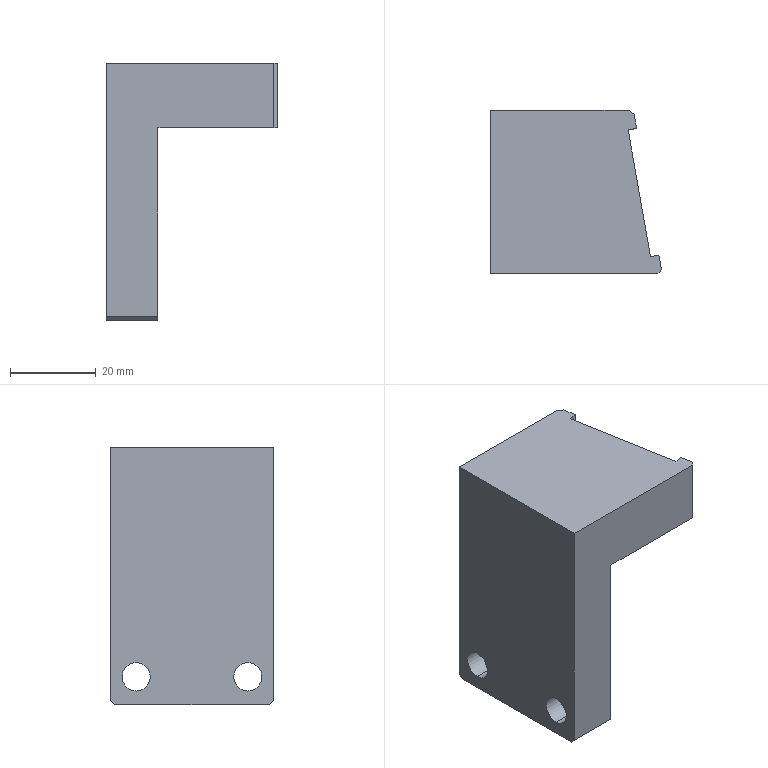Part | SolidWorks | features BaseBody 1 | 1 solid | 30 faces | box 39.85 x 38 x 60 mm | volume 38628 mm3 | plane 18 | cylinder 10 | cone 2 | commonest cylinder face diameters 6.6 x4 11 x4 5 x2
STEP:
#1=CARTESIAN_POINT('',(0.,6.,-56.8));
#2=VERTEX_POINT('',#1);
#3=CARTESIAN_POINT('',(0.,6.,-50.2));
#4=VERTEX_POINT('',#3);
#5=CARTESIAN_POINT('',(0.,6.,-53.5));
#6=DIRECTION('',(-1.,0.,0.));
#7=DIRECTION('',(0.,0.,-1.));
#8=AXIS2_PLACEMENT_3D('',#5,#6,#7);
#9=CIRCLE('',#8,3.3);
#10=EDGE_CURVE('',#2,#4,#9,.T.);
#11=ORIENTED_EDGE('',*,*,#10,.T.);
#12=CARTESIAN_POINT('',(6.,6.,-50.2));
#13=VERTEX_POINT('',#12);
#14=CARTESIAN_POINT('',(12.,6.,-50.2));
#15=DIRECTION('',(1.,0.,0.));
#16=VECTOR('',#15,1000.);
#17=LINE('',#14,#16);
#18=EDGE_CURVE('',#4,#13,#17,.T.);
#19=ORIENTED_EDGE('',*,*,#18,.T.);
#20=CARTESIAN_POINT('',(6.,6.,-56.8));
#21=VERTEX_POINT('',#20);
#22=CARTESIAN_POINT('',(6.,6.,-53.5));
#23=DIRECTION('',(-1.,0.,0.));
#24=DIRECTION('',(0.,0.,-1.));
#25=AXIS2_PLACEMENT_3D('',#22,#23,#24);
#26=CIRCLE('',#25,3.3);
#27=EDGE_CURVE('',#21,#13,#26,.T.);
#28=ORIENTED_EDGE('',*,*,#27,.F.);
#29=CARTESIAN_POINT('',(12.,6.,-56.8));
#30=DIRECTION('',(1.,0.,0.));
#31=VECTOR('',#30,1000.);
#32=LINE('',#29,#31);
#33=EDGE_CURVE('',#2,#21,#32,.T.);
#34=ORIENTED_EDGE('',*,*,#33,.F.);
#35=EDGE_LOOP('',(#11,#19,#28,#34));
#36=FACE_OUTER_BOUND('',#35,.T.);
#37=CARTESIAN_POINT('',(12.,6.,-53.5));
#38=DIRECTION('',(1.,0.,0.));
#39=DIRECTION('',(0.,0.,-1.));
#40=AXIS2_PLACEMENT_3D('',#37,#38,#39);
#41=CYLINDRICAL_SURFACE('',#40,3.3);
#42=ADVANCED_FACE('',(#36),#41,.F.);
#43=CARTESIAN_POINT('',(0.,32.,-56.8));
#44=VERTEX_POINT('',#43);
#45=CARTESIAN_POINT('',(0.,32.,-50.2));
#46=VERTEX_POINT('',#45);
#47=CARTESIAN_POINT('',(0.,32.,-53.5));
#48=DIRECTION('',(-1.,0.,0.));
#49=DIRECTION('',(0.,0.,-1.));
#50=AXIS2_PLACEMENT_3D('',#47,#48,#49);
#51=CIRCLE('',#50,3.3);
#52=EDGE_CURVE('',#44,#46,#51,.T.);
#53=ORIENTED_EDGE('',*,*,#52,.T.);
#54=CARTESIAN_POINT('',(6.,32.,-50.2));
#55=VERTEX_POINT('',#54);
#56=CARTESIAN_POINT('',(12.,32.,-50.2));
#57=DIRECTION('',(1.,0.,0.));
#58=VECTOR('',#57,1000.);
#59=LINE('',#56,#58);
#60=EDGE_CURVE('',#46,#55,#59,.T.);
#61=ORIENTED_EDGE('',*,*,#60,.T.);
#62=CARTESIAN_POINT('',(6.,32.,-56.8));
#63=VERTEX_POINT('',#62);
#64=CARTESIAN_POINT('',(6.,32.,-53.5));
#65=DIRECTION('',(-1.,0.,0.));
#66=DIRECTION('',(0.,0.,-1.));
#67=AXIS2_PLACEMENT_3D('',#64,#65,#66);
#68=CIRCLE('',#67,3.3);
#69=EDGE_CURVE('',#63,#55,#68,.T.);
#70=ORIENTED_EDGE('',*,*,#69,.F.);
#71=CARTESIAN_POINT('',(12.,32.,-56.8));
#72=DIRECTION('',(1.,0.,0.));
#73=VECTOR('',#72,1000.);
#74=LINE('',#71,#73);
#75=EDGE_CURVE('',#44,#63,#74,.T.);
#76=ORIENTED_EDGE('',*,*,#75,.F.);
#77=EDGE_LOOP('',(#53,#61,#70,#76));
#78=FACE_OUTER_BOUND('',#77,.T.);
#79=CARTESIAN_POINT('',(12.,32.,-53.5));
#80=DIRECTION('',(1.,0.,0.));
#81=DIRECTION('',(0.,0.,-1.));
#82=AXIS2_PLACEMENT_3D('',#79,#80,#81);
#83=CYLINDRICAL_SURFACE('',#82,3.3);
#84=ADVANCED_FACE('',(#78),#83,.F.);
#85=CARTESIAN_POINT('',(6.,6.,-59.));
#86=VERTEX_POINT('',#85);
#87=CARTESIAN_POINT('',(6.,6.,-48.));
#88=VERTEX_POINT('',#87);
#89=CARTESIAN_POINT('',(6.,6.,-53.5));
#90=DIRECTION('',(-1.,0.,0.));
#91=DIRECTION('',(0.,0.,-1.));
#92=AXIS2_PLACEMENT_3D('',#89,#90,#91);
#93=CIRCLE('',#92,5.5);
#94=EDGE_CURVE('',#86,#88,#93,.T.);
#95=ORIENTED_EDGE('',*,*,#94,.T.);
#96=CARTESIAN_POINT('',(12.,6.,-48.));
#97=VERTEX_POINT('',#96);
#98=CARTESIAN_POINT('',(12.,6.,-48.));
#99=DIRECTION('',(1.,0.,0.));
#100=VECTOR('',#99,1000.);
#101=LINE('',#98,#100);
#102=EDGE_CURVE('',#88,#97,#101,.T.);
#103=ORIENTED_EDGE('',*,*,#102,.T.);
#104=CARTESIAN_POINT('',(12.,6.,-59.));
#105=VERTEX_POINT('',#104);
#106=CARTESIAN_POINT('',(12.,6.,-53.5));
#107=DIRECTION('',(1.,0.,0.));
#108=DIRECTION('',(0.,0.,-1.));
#109=AXIS2_PLACEMENT_3D('',#106,#107,#108);
#110=CIRCLE('',#109,5.5);
#111=EDGE_CURVE('',#97,#105,#110,.T.);
#112=ORIENTED_EDGE('',*,*,#111,.T.);
#113=CARTESIAN_POINT('',(12.,6.,-59.));
#114=DIRECTION('',(1.,0.,0.));
#115=VECTOR('',#114,1000.);
#116=LINE('',#113,#115);
#117=EDGE_CURVE('',#86,#105,#116,.T.);
#118=ORIENTED_EDGE('',*,*,#117,.F.);
#119=EDGE_LOOP('',(#95,#103,#112,#118));
#120=FACE_OUTER_BOUND('',#119,.T.);
#121=CARTESIAN_POINT('',(12.,6.,-53.5));
#122=DIRECTION('',(1.,0.,0.));
#123=DIRECTION('',(0.,0.,-1.));
#124=AXIS2_PLACEMENT_3D('',#121,#122,#123);
#125=CYLINDRICAL_SURFACE('',#124,5.5);
#126=ADVANCED_FACE('',(#120),#125,.F.);
#127=CARTESIAN_POINT('',(6.,32.,-59.));
#128=VERTEX_POINT('',#127);
#129=CARTESIAN_POINT('',(6.,32.,-48.));
#130=VERTEX_POINT('',#129);
#131=CARTESIAN_POINT('',(6.,32.,-53.5));
#132=DIRECTION('',(-1.,0.,0.));
#133=DIRECTION('',(0.,0.,-1.));
#134=AXIS2_PLACEMENT_3D('',#131,#132,#133);
#135=CIRCLE('',#134,5.5);
#136=EDGE_CURVE('',#128,#130,#135,.T.);
#137=ORIENTED_EDGE('',*,*,#136,.T.);
#138=CARTESIAN_POINT('',(12.,32.,-48.));
#139=VERTEX_POINT('',#138);
#140=CARTESIAN_POINT('',(12.,32.,-48.));
#141=DIRECTION('',(1.,0.,0.));
#142=VECTOR('',#141,1000.);
#143=LINE('',#140,#142);
#144=EDGE_CURVE('',#130,#139,#143,.T.);
#145=ORIENTED_EDGE('',*,*,#144,.T.);
#146=CARTESIAN_POINT('',(12.,32.,-59.));
#147=VERTEX_POINT('',#146);
#148=CARTESIAN_POINT('',(12.,32.,-53.5));
#149=DIRECTION('',(1.,0.,0.));
#150=DIRECTION('',(0.,0.,-1.));
#151=AXIS2_PLACEMENT_3D('',#148,#149,#150);
#152=CIRCLE('',#151,5.5);
#153=EDGE_CURVE('',#139,#147,#152,.T.);
#154=ORIENTED_EDGE('',*,*,#153,.T.);
#155=CARTESIAN_POINT('',(12.,32.,-59.));
#156=DIRECTION('',(1.,0.,0.));
#157=VECTOR('',#156,1000.);
#158=LINE('',#155,#157);
#159=EDGE_CURVE('',#128,#147,#158,.T.);
#160=ORIENTED_EDGE('',*,*,#159,.F.);
#161=EDGE_LOOP('',(#137,#145,#154,#160));
#162=FACE_OUTER_BOUND('',#161,.T.);
#163=CARTESIAN_POINT('',(12.,32.,-53.5));
#164=DIRECTION('',(1.,0.,0.));
#165=DIRECTION('',(0.,0.,-1.));
#166=AXIS2_PLACEMENT_3D('',#163,#164,#165);
#167=CYLINDRICAL_SURFACE('',#166,5.5);
#168=ADVANCED_FACE('',(#162),#167,.F.);
#169=CARTESIAN_POINT('',(20.342,13.586,-7.5));
#170=VERTEX_POINT('',#169);
#171=CARTESIAN_POINT('',(19.474,18.51,-7.5));
#172=VERTEX_POINT('',#171);
#173=CARTESIAN_POINT('',(19.908,16.048,-7.5));
#174=DIRECTION('',(0.9848,0.1736,0.));
#175=DIRECTION('',(-0.1736,0.9848,0.));
#176=AXIS2_PLACEMENT_3D('',#173,#174,#175);
#177=CIRCLE('',#176,2.5);
#178=EDGE_CURVE('',#170,#172,#177,.T.);
#179=ORIENTED_EDGE('',*,*,#178,.F.);
#180=CARTESIAN_POINT('',(35.114,16.191,-7.5));
#181=VERTEX_POINT('',#180);
#182=CARTESIAN_POINT('',(35.114,16.191,-7.5));
#183=DIRECTION('',(0.9848,0.1736,0.));
#184=VECTOR('',#183,1000.);
#185=LINE('',#182,#184);
#186=EDGE_CURVE('',#170,#181,#185,.T.);
#187=ORIENTED_EDGE('',*,*,#186,.T.);
#188=CARTESIAN_POINT('',(34.246,21.115,-7.5));
#189=VERTEX_POINT('',#188);
#190=CARTESIAN_POINT('',(34.68,18.653,-7.5));
#191=DIRECTION('',(-0.9848,-0.1736,0.));
#192=DIRECTION('',(-0.1736,0.9848,0.));
#193=AXIS2_PLACEMENT_3D('',#190,#191,#192);
#194=CIRCLE('',#193,2.5);
#195=EDGE_CURVE('',#189,#181,#194,.T.);
#196=ORIENTED_EDGE('',*,*,#195,.F.);
#197=CARTESIAN_POINT('',(34.246,21.115,-7.5));
#198=DIRECTION('',(0.9848,0.1736,0.));
#199=VECTOR('',#198,1000.);
#200=LINE('',#197,#199);
#201=EDGE_CURVE('',#172,#189,#200,.T.);
#202=ORIENTED_EDGE('',*,*,#201,.F.);
#203=EDGE_LOOP('',(#179,#187,#196,#202));
#204=FACE_OUTER_BOUND('',#203,.T.);
#205=CARTESIAN_POINT('',(34.68,18.653,-7.5));
#206=DIRECTION('',(0.9848,0.1736,0.));
#207=DIRECTION('',(-0.1736,0.9848,0.));
#208=AXIS2_PLACEMENT_3D('',#205,#206,#207);
#209=CYLINDRICAL_SURFACE('',#208,2.5);
#210=ADVANCED_FACE('',(#204),#209,.F.);
#211=CARTESIAN_POINT('',(18.429,15.787,-7.5));
#212=VERTEX_POINT('',#211);
#213=CARTESIAN_POINT('',(19.474,18.51,-7.5));
#214=DIRECTION('',(0.3584,0.9336,0.));
#215=VECTOR('',#214,1000.);
#216=LINE('',#213,#215);
#217=EDGE_CURVE('',#212,#172,#216,.T.);
#218=ORIENTED_EDGE('',*,*,#217,.F.);
#219=CARTESIAN_POINT('',(20.342,13.586,-7.5));
#220=DIRECTION('',(0.6561,-0.7547,0.));
#221=VECTOR('',#220,1000.);
#222=LINE('',#219,#221);
#223=EDGE_CURVE('',#212,#170,#222,.T.);
#224=ORIENTED_EDGE('',*,*,#223,.T.);
#225=ORIENTED_EDGE('',*,*,#178,.T.);
#226=EDGE_LOOP('',(#218,#224,#225));
#227=FACE_OUTER_BOUND('',#226,.T.);
#228=CARTESIAN_POINT('',(19.908,16.048,-7.5));
#229=DIRECTION('',(0.9848,0.1736,0.));
#230=DIRECTION('',(-0.1736,0.9848,0.));
#231=AXIS2_PLACEMENT_3D('',#228,#229,#230);
#232=CONICAL_SURFACE('',#231,2.5,1.03);
#233=ADVANCED_FACE('',(#227),#232,.F.);
#234=CARTESIAN_POINT('',(0.,38.,-59.));
#235=VERTEX_POINT('',#234);
#236=CARTESIAN_POINT('',(0.,37.,-60.));
#237=VERTEX_POINT('',#236);
#238=CARTESIAN_POINT('',(0.,38.,-59.));
#239=DIRECTION('',(0.,-0.7071,-0.7071));
#240=VECTOR('',#239,1000.);
#241=LINE('',#238,#240);
#242=EDGE_CURVE('',#235,#237,#241,.T.);
#243=ORIENTED_EDGE('',*,*,#242,.T.);
#244=CARTESIAN_POINT('',(0.,1.,-60.));
#245=VERTEX_POINT('',#244);
#246=CARTESIAN_POINT('',(0.,38.,-60.));
#247=DIRECTION('',(0.,1.,0.));
#248=VECTOR('',#247,1000.);
#249=LINE('',#246,#248);
#250=EDGE_CURVE('',#245,#237,#249,.T.);
#251=ORIENTED_EDGE('',*,*,#250,.F.);
#252=CARTESIAN_POINT('',(0.,0.,-59.));
#253=VERTEX_POINT('',#252);
#254=CARTESIAN_POINT('',(0.,1.,-60.));
#255=DIRECTION('',(0.,0.7071,-0.7071));
#256=VECTOR('',#255,1000.);
#257=LINE('',#254,#256);
#258=EDGE_CURVE('',#253,#245,#257,.T.);
#259=ORIENTED_EDGE('',*,*,#258,.F.);
#260=CARTESIAN_POINT('',(0.,0.,0.));
#261=VERTEX_POINT('',#260);
#262=CARTESIAN_POINT('',(0.,0.,0.));
#263=DIRECTION('',(0.,0.,-1.));
#264=VECTOR('',#263,1000.);
#265=LINE('',#262,#264);
#266=EDGE_CURVE('',#261,#253,#265,.T.);
#267=ORIENTED_EDGE('',*,*,#266,.F.);
#268=CARTESIAN_POINT('',(0.,38.,0.));
#269=VERTEX_POINT('',#268);
#270=CARTESIAN_POINT('',(0.,38.,0.));
#271=DIRECTION('',(0.,-1.,0.));
#272=VECTOR('',#271,1000.);
#273=LINE('',#270,#272);
#274=EDGE_CURVE('',#269,#261,#273,.T.);
#275=ORIENTED_EDGE('',*,*,#274,.F.);
#276=CARTESIAN_POINT('',(0.,38.,0.));
#277=DIRECTION('',(0.,0.,1.));
#278=VECTOR('',#277,1000.);
#279=LINE('',#276,#278);
#280=EDGE_CURVE('',#235,#269,#279,.T.);
#281=ORIENTED_EDGE('',*,*,#280,.F.);
#282=EDGE_LOOP('',(#243,#251,#259,#267,#275,#281));
#283=FACE_OUTER_BOUND('',#282,.T.);
#284=ORIENTED_EDGE('',*,*,#10,.F.);
#285=CARTESIAN_POINT('',(0.,6.,-53.5));
#286=DIRECTION('',(-1.,0.,0.));
#287=DIRECTION('',(0.,0.,-1.));
#288=AXIS2_PLACEMENT_3D('',#285,#286,#287);
#289=CIRCLE('',#288,3.3);
#290=EDGE_CURVE('',#4,#2,#289,.T.);
#291=ORIENTED_EDGE('',*,*,#290,.F.);
#292=EDGE_LOOP('',(#284,#291));
#293=FACE_BOUND('',#292,.T.);
#294=ORIENTED_EDGE('',*,*,#52,.F.);
#295=CARTESIAN_POINT('',(0.,32.,-53.5));
#296=DIRECTION('',(-1.,0.,0.));
#297=DIRECTION('',(0.,0.,-1.));
#298=AXIS2_PLACEMENT_3D('',#295,#296,#297);
#299=CIRCLE('',#298,3.3);
#300=EDGE_CURVE('',#46,#44,#299,.T.);
#301=ORIENTED_EDGE('',*,*,#300,.F.);
#302=EDGE_LOOP('',(#294,#301));
#303=FACE_BOUND('',#302,.T.);
#304=CARTESIAN_POINT('',(0.,38.,0.));
#305=DIRECTION('',(1.,0.,0.));
#306=DIRECTION('',(0.,0.,-1.));
#307=AXIS2_PLACEMENT_3D('',#304,#305,#306);
#308=PLANE('',#307);
#309=ADVANCED_FACE('',(#283,#293,#303),#308,.F.);
#310=CARTESIAN_POINT('',(12.,38.,-59.));
#311=VERTEX_POINT('',#310);
#312=CARTESIAN_POINT('',(0.,38.,-59.));
#313=DIRECTION('',(1.,0.,0.));
#314=VECTOR('',#313,1000.);
#315=LINE('',#312,#314);
#316=EDGE_CURVE('',#235,#311,#315,.T.);
#317=ORIENTED_EDGE('',*,*,#316,.F.);
#318=ORIENTED_EDGE('',*,*,#280,.T.);
#319=CARTESIAN_POINT('',(32.067,38.,0.));
#320=VERTEX_POINT('',#319);
#321=CARTESIAN_POINT('',(0.,38.,0.));
#322=DIRECTION('',(-1.,0.,0.));
#323=VECTOR('',#322,1000.);
#324=LINE('',#321,#323);
#325=EDGE_CURVE('',#320,#269,#324,.T.);
#326=ORIENTED_EDGE('',*,*,#325,.F.);
#327=CARTESIAN_POINT('',(32.067,38.,-15.));
#328=VERTEX_POINT('',#327);
#329=CARTESIAN_POINT('',(32.067,38.,0.));
#330=DIRECTION('',(0.,0.,1.));
#331=VECTOR('',#330,1000.);
#332=LINE('',#329,#331);
#333=EDGE_CURVE('',#328,#320,#332,.T.);
#334=ORIENTED_EDGE('',*,*,#333,.F.);
#335=CARTESIAN_POINT('',(12.,38.,-15.));
#336=VERTEX_POINT('',#335);
#337=CARTESIAN_POINT('',(0.,38.,-15.));
#338=DIRECTION('',(1.,0.,0.));
#339=VECTOR('',#338,1000.);
#340=LINE('',#337,#339);
#341=EDGE_CURVE('',#336,#328,#340,.T.);
#342=ORIENTED_EDGE('',*,*,#341,.F.);
#343=CARTESIAN_POINT('',(12.,38.,0.));
#344=DIRECTION('',(0.,0.,1.));
#345=VECTOR('',#344,1000.);
#346=LINE('',#343,#345);
#347=EDGE_CURVE('',#311,#336,#346,.T.);
#348=ORIENTED_EDGE('',*,*,#347,.F.);
#349=EDGE_LOOP('',(#317,#318,#326,#334,#342,#348));
#350=FACE_OUTER_BOUND('',#349,.T.);
#351=CARTESIAN_POINT('',(0.,38.,0.));
#352=DIRECTION('',(0.,-1.,0.));
#353=DIRECTION('',(0.,0.,-1.));
#354=AXIS2_PLACEMENT_3D('',#351,#352,#353);
#355=PLANE('',#354);
#356=ADVANCED_FACE('',(#350),#355,.F.);
#357=CARTESIAN_POINT('',(12.,37.,-60.));
#358=VERTEX_POINT('',#357);
#359=CARTESIAN_POINT('',(0.,37.,-60.));
#360=DIRECTION('',(-1.,0.,0.));
#361=VECTOR('',#360,1000.);
#362=LINE('',#359,#361);
#363=EDGE_CURVE('',#358,#237,#362,.T.);
#364=ORIENTED_EDGE('',*,*,#363,.F.);
#365=CARTESIAN_POINT('',(12.,1.,-60.));
#366=VERTEX_POINT('',#365);
#367=CARTESIAN_POINT('',(12.,38.,-60.));
#368=DIRECTION('',(0.,1.,0.));
#369=VECTOR('',#368,1000.);
#370=LINE('',#367,#369);
#371=EDGE_CURVE('',#366,#358,#370,.T.);
#372=ORIENTED_EDGE('',*,*,#371,.F.);
#373=CARTESIAN_POINT('',(0.,1.,-60.));
#374=DIRECTION('',(1.,0.,0.));
#375=VECTOR('',#374,1000.);
#376=LINE('',#373,#375);
#377=EDGE_CURVE('',#245,#366,#376,.T.);
#378=ORIENTED_EDGE('',*,*,#377,.F.);
#379=ORIENTED_EDGE('',*,*,#250,.T.);
#380=EDGE_LOOP('',(#364,#372,#378,#379));
#381=FACE_OUTER_BOUND('',#380,.T.);
#382=CARTESIAN_POINT('',(0.,38.,-60.));
#383=DIRECTION('',(0.,0.,1.));
#384=DIRECTION('',(1.,0.,0.));
#385=AXIS2_PLACEMENT_3D('',#382,#383,#384);
#386=PLANE('',#385);
#387=ADVANCED_FACE('',(#381),#386,.F.);
#388=CARTESIAN_POINT('',(39.,0.,-15.));
#389=VERTEX_POINT('',#388);
#390=CARTESIAN_POINT('',(39.,0.,0.));
#391=VERTEX_POINT('',#390);
#392=CARTESIAN_POINT('',(39.,0.,0.));
#393=DIRECTION('',(0.,0.,1.));
#394=VECTOR('',#393,1000.);
#395=LINE('',#392,#394);
#396=EDGE_CURVE('',#389,#391,#395,.T.);
#397=ORIENTED_EDGE('',*,*,#396,.T.);
#398=CARTESIAN_POINT('',(0.,0.,0.));
#399=DIRECTION('',(-1.,0.,0.));
#400=VECTOR('',#399,1000.);
#401=LINE('',#398,#400);
#402=EDGE_CURVE('',#391,#261,#401,.T.);
#403=ORIENTED_EDGE('',*,*,#402,.T.);
#404=ORIENTED_EDGE('',*,*,#266,.T.);
#405=CARTESIAN_POINT('',(12.,0.,-59.));
#406=VERTEX_POINT('',#405);
#407=CARTESIAN_POINT('',(0.,0.,-59.));
#408=DIRECTION('',(1.,0.,0.));
#409=VECTOR('',#408,1000.);
#410=LINE('',#407,#409);
#411=EDGE_CURVE('',#253,#406,#410,.T.);
#412=ORIENTED_EDGE('',*,*,#411,.T.);
#413=CARTESIAN_POINT('',(12.,0.,-15.));
#414=VERTEX_POINT('',#413);
#415=CARTESIAN_POINT('',(12.,0.,0.));
#416=DIRECTION('',(0.,0.,1.));
#417=VECTOR('',#416,1000.);
#418=LINE('',#415,#417);
#419=EDGE_CURVE('',#406,#414,#418,.T.);
#420=ORIENTED_EDGE('',*,*,#419,.T.);
#421=CARTESIAN_POINT('',(0.,0.,-15.));
#422=DIRECTION('',(1.,0.,0.));
#423=VECTOR('',#422,1000.);
#424=LINE('',#421,#423);
#425=EDGE_CURVE('',#414,#389,#424,.T.);
#426=ORIENTED_EDGE('',*,*,#425,.T.);
#427=EDGE_LOOP('',(#397,#403,#404,#412,#420,#426));
#428=FACE_OUTER_BOUND('',#427,.T.);
#429=CARTESIAN_POINT('',(0.,0.,0.));
#430=DIRECTION('',(0.,-1.,0.));
#431=DIRECTION('',(0.,0.,-1.));
#432=AXIS2_PLACEMENT_3D('',#429,#430,#431);
#433=PLANE('',#432);
#434=ADVANCED_FACE('',(#428),#433,.T.);
#435=CARTESIAN_POINT('',(39.85,0.8501,0.));
#436=VERTEX_POINT('',#435);
#437=CARTESIAN_POINT('',(39.85,0.8501,0.));
#438=DIRECTION('',(-0.7071,-0.7071,0.));
#439=VECTOR('',#438,1000.);
#440=LINE('',#437,#439);
#441=EDGE_CURVE('',#436,#391,#440,.T.);
#442=ORIENTED_EDGE('',*,*,#441,.F.);
#443=CARTESIAN_POINT('',(39.255,4.228,0.));
#444=VERTEX_POINT('',#443);
#445=CARTESIAN_POINT('',(39.255,4.228,0.));
#446=DIRECTION('',(0.1736,-0.9848,0.));
#447=VECTOR('',#446,1000.);
#448=LINE('',#445,#447);
#449=EDGE_CURVE('',#444,#436,#448,.T.);
#450=ORIENTED_EDGE('',*,*,#449,.F.);
#451=CARTESIAN_POINT('',(37.285,3.881,0.));
#452=VERTEX_POINT('',#451);
#453=CARTESIAN_POINT('',(37.285,3.881,0.));
#454=DIRECTION('',(0.9848,0.1736,0.));
#455=VECTOR('',#454,1000.);
#456=LINE('',#453,#455);
#457=EDGE_CURVE('',#452,#444,#456,.T.);
#458=ORIENTED_EDGE('',*,*,#457,.F.);
#459=CARTESIAN_POINT('',(32.075,33.425,0.));
#460=VERTEX_POINT('',#459);
#461=CARTESIAN_POINT('',(32.075,33.425,0.));
#462=DIRECTION('',(0.1736,-0.9848,0.));
#463=VECTOR('',#462,1000.);
#464=LINE('',#461,#463);
#465=EDGE_CURVE('',#460,#452,#464,.T.);
#466=ORIENTED_EDGE('',*,*,#465,.F.);
#467=CARTESIAN_POINT('',(34.045,33.772,0.));
#468=VERTEX_POINT('',#467);
#469=CARTESIAN_POINT('',(34.045,33.772,0.));
#470=DIRECTION('',(-0.9848,-0.1736,0.));
#471=VECTOR('',#470,1000.);
#472=LINE('',#469,#471);
#473=EDGE_CURVE('',#468,#460,#472,.T.);
#474=ORIENTED_EDGE('',*,*,#473,.F.);
#475=CARTESIAN_POINT('',(33.473,37.015,0.));
#476=VERTEX_POINT('',#475);
#477=CARTESIAN_POINT('',(33.473,37.015,0.));
#478=DIRECTION('',(0.1736,-0.9848,0.));
#479=VECTOR('',#478,1000.);
#480=LINE('',#477,#479);
#481=EDGE_CURVE('',#476,#468,#480,.T.);
#482=ORIENTED_EDGE('',*,*,#481,.F.);
#483=CARTESIAN_POINT('',(32.067,38.,0.));
#484=DIRECTION('',(0.8192,-0.5736,0.));
#485=VECTOR('',#484,1000.);
#486=LINE('',#483,#485);
#487=EDGE_CURVE('',#320,#476,#486,.T.);
#488=ORIENTED_EDGE('',*,*,#487,.F.);
#489=ORIENTED_EDGE('',*,*,#325,.T.);
#490=ORIENTED_EDGE('',*,*,#274,.T.);
#491=ORIENTED_EDGE('',*,*,#402,.F.);
#492=EDGE_LOOP('',(#442,#450,#458,#466,#474,#482,#488,#489,#490,#491));
#493=FACE_OUTER_BOUND('',#492,.T.);
#494=CARTESIAN_POINT('',(40.,38.,0.));
#495=DIRECTION('',(0.,0.,-1.));
#496=DIRECTION('',(-1.,0.,0.));
#497=AXIS2_PLACEMENT_3D('',#494,#495,#496);
#498=PLANE('',#497);
#499=ADVANCED_FACE('',(#493),#498,.F.);
#500=ORIENTED_EDGE('',*,*,#18,.F.);
#501=ORIENTED_EDGE('',*,*,#290,.T.);
#502=ORIENTED_EDGE('',*,*,#33,.T.);
#503=CARTESIAN_POINT('',(6.,6.,-53.5));
#504=DIRECTION('',(-1.,0.,0.));
#505=DIRECTION('',(0.,0.,-1.));
#506=AXIS2_PLACEMENT_3D('',#503,#504,#505);
#507=CIRCLE('',#506,3.3);
#508=EDGE_CURVE('',#13,#21,#507,.T.);
#509=ORIENTED_EDGE('',*,*,#508,.F.);
#510=EDGE_LOOP('',(#500,#501,#502,#509));
#511=FACE_OUTER_BOUND('',#510,.T.);
#512=CARTESIAN_POINT('',(12.,6.,-53.5));
#513=DIRECTION('',(1.,0.,0.));
#514=DIRECTION('',(0.,0.,-1.));
#515=AXIS2_PLACEMENT_3D('',#512,#513,#514);
#516=CYLINDRICAL_SURFACE('',#515,3.3);
#517=ADVANCED_FACE('',(#511),#516,.F.);
#518=ORIENTED_EDGE('',*,*,#60,.F.);
#519=ORIENTED_EDGE('',*,*,#300,.T.);
#520=ORIENTED_EDGE('',*,*,#75,.T.);
#521=CARTESIAN_POINT('',(6.,32.,-53.5));
#522=DIRECTION('',(-1.,0.,0.));
#523=DIRECTION('',(0.,0.,-1.));
#524=AXIS2_PLACEMENT_3D('',#521,#522,#523);
#525=CIRCLE('',#524,3.3);
#526=EDGE_CURVE('',#55,#63,#525,.T.);
#527=ORIENTED_EDGE('',*,*,#526,.F.);
#528=EDGE_LOOP('',(#518,#519,#520,#527));
#529=FACE_OUTER_BOUND('',#528,.T.);
#530=CARTESIAN_POINT('',(12.,32.,-53.5));
#531=DIRECTION('',(1.,0.,0.));
#532=DIRECTION('',(0.,0.,-1.));
#533=AXIS2_PLACEMENT_3D('',#530,#531,#532);
#534=CYLINDRICAL_SURFACE('',#533,3.3);
#535=ADVANCED_FACE('',(#529),#534,.F.);
#536=CARTESIAN_POINT('',(12.,38.,-59.));
#537=DIRECTION('',(0.,-0.7071,-0.7071));
#538=VECTOR('',#537,1000.);
#539=LINE('',#536,#538);
#540=EDGE_CURVE('',#311,#358,#539,.T.);
#541=ORIENTED_EDGE('',*,*,#540,.F.);
#542=ORIENTED_EDGE('',*,*,#347,.T.);
#543=CARTESIAN_POINT('',(12.,38.,-15.));
#544=DIRECTION('',(0.,1.,0.));
#545=VECTOR('',#544,1000.);
#546=LINE('',#543,#545);
#547=EDGE_CURVE('',#414,#336,#546,.T.);
#548=ORIENTED_EDGE('',*,*,#547,.F.);
#549=ORIENTED_EDGE('',*,*,#419,.F.);
#550=CARTESIAN_POINT('',(12.,1.,-60.));
#551=DIRECTION('',(0.,-0.7071,0.7071));
#552=VECTOR('',#551,1000.);
#553=LINE('',#550,#552);
#554=EDGE_CURVE('',#366,#406,#553,.T.);
#555=ORIENTED_EDGE('',*,*,#554,.F.);
#556=ORIENTED_EDGE('',*,*,#371,.T.);
#557=EDGE_LOOP('',(#541,#542,#548,#549,#555,#556));
#558=FACE_OUTER_BOUND('',#557,.T.);
#559=CARTESIAN_POINT('',(12.,6.,-53.5));
#560=DIRECTION('',(1.,0.,0.));
#561=DIRECTION('',(0.,0.,-1.));
#562=AXIS2_PLACEMENT_3D('',#559,#560,#561);
#563=CIRCLE('',#562,5.5);
#564=EDGE_CURVE('',#105,#97,#563,.T.);
#565=ORIENTED_EDGE('',*,*,#564,.F.);
#566=ORIENTED_EDGE('',*,*,#111,.F.);
#567=EDGE_LOOP('',(#565,#566));
#568=FACE_BOUND('',#567,.T.);
#569=CARTESIAN_POINT('',(12.,32.,-53.5));
#570=DIRECTION('',(1.,0.,0.));
#571=DIRECTION('',(0.,0.,-1.));
#572=AXIS2_PLACEMENT_3D('',#569,#570,#571);
#573=CIRCLE('',#572,5.5);
#574=EDGE_CURVE('',#147,#139,#573,.T.);
#575=ORIENTED_EDGE('',*,*,#574,.F.);
#576=ORIENTED_EDGE('',*,*,#153,.F.);
#577=EDGE_LOOP('',(#575,#576));
#578=FACE_BOUND('',#577,.T.);
#579=CARTESIAN_POINT('',(12.,38.,-60.));
#580=DIRECTION('',(-1.,0.,0.));
#581=DIRECTION('',(0.,0.,1.));
#582=AXIS2_PLACEMENT_3D('',#579,#580,#581);
#583=PLANE('',#582);
#584=ADVANCED_FACE('',(#558,#568,#578),#583,.F.);
#585=ORIENTED_EDGE('',*,*,#363,.T.);
#586=ORIENTED_EDGE('',*,*,#242,.F.);
#587=ORIENTED_EDGE('',*,*,#316,.T.);
#588=ORIENTED_EDGE('',*,*,#540,.T.);
#589=EDGE_LOOP('',(#585,#586,#587,#588));
#590=FACE_OUTER_BOUND('',#589,.T.);
#591=CARTESIAN_POINT('',(0.,38.,-59.));
#592=DIRECTION('',(0.,-0.7071,0.7071));
#593=DIRECTION('',(0.,-0.7071,-0.7071));
#594=AXIS2_PLACEMENT_3D('',#591,#592,#593);
#595=PLANE('',#594);
#596=ADVANCED_FACE('',(#590),#595,.F.);
#597=CARTESIAN_POINT('',(33.473,37.015,-15.));
#598=VERTEX_POINT('',#597);
#599=CARTESIAN_POINT('',(33.473,37.015,0.));
#600=DIRECTION('',(0.,0.,1.));
#601=VECTOR('',#600,1000.);
#602=LINE('',#599,#601);
#603=EDGE_CURVE('',#598,#476,#602,.T.);
#604=ORIENTED_EDGE('',*,*,#603,.F.);
#605=CARTESIAN_POINT('',(32.067,38.,-15.));
#606=DIRECTION('',(0.8192,-0.5736,0.));
#607=VECTOR('',#606,1000.);
#608=LINE('',#605,#607);
#609=EDGE_CURVE('',#328,#598,#608,.T.);
#610=ORIENTED_EDGE('',*,*,#609,.F.);
#611=ORIENTED_EDGE('',*,*,#333,.T.);
#612=ORIENTED_EDGE('',*,*,#487,.T.);
#613=EDGE_LOOP('',(#604,#610,#611,#612));
#614=FACE_OUTER_BOUND('',#613,.T.);
#615=CARTESIAN_POINT('',(32.067,38.,0.));
#616=DIRECTION('',(-0.5736,-0.8192,0.));
#617=DIRECTION('',(0.8192,-0.5736,0.));
#618=AXIS2_PLACEMENT_3D('',#615,#616,#617);
#619=PLANE('',#618);
#620=ADVANCED_FACE('',(#614),#619,.F.);
#621=CARTESIAN_POINT('',(39.85,0.8501,-15.));
#622=VERTEX_POINT('',#621);
#623=CARTESIAN_POINT('',(39.,0.,-15.));
#624=DIRECTION('',(0.7071,0.7071,0.));
#625=VECTOR('',#624,1000.);
#626=LINE('',#623,#625);
#627=EDGE_CURVE('',#389,#622,#626,.T.);
#628=ORIENTED_EDGE('',*,*,#627,.F.);
#629=ORIENTED_EDGE('',*,*,#425,.F.);
#630=ORIENTED_EDGE('',*,*,#547,.T.);
#631=ORIENTED_EDGE('',*,*,#341,.T.);
#632=ORIENTED_EDGE('',*,*,#609,.T.);
#633=CARTESIAN_POINT('',(34.045,33.772,-15.));
#634=VERTEX_POINT('',#633);
#635=CARTESIAN_POINT('',(34.045,33.772,-15.));
#636=DIRECTION('',(-0.1736,0.9848,0.));
#637=VECTOR('',#636,1000.);
#638=LINE('',#635,#637);
#639=EDGE_CURVE('',#634,#598,#638,.T.);
#640=ORIENTED_EDGE('',*,*,#639,.F.);
#641=CARTESIAN_POINT('',(32.075,33.425,-15.));
#642=VERTEX_POINT('',#641);
#643=CARTESIAN_POINT('',(32.075,33.425,-15.));
#644=DIRECTION('',(0.9848,0.1736,0.));
#645=VECTOR('',#644,1000.);
#646=LINE('',#643,#645);
#647=EDGE_CURVE('',#642,#634,#646,.T.);
#648=ORIENTED_EDGE('',*,*,#647,.F.);
#649=CARTESIAN_POINT('',(37.285,3.881,-15.));
#650=VERTEX_POINT('',#649);
#651=CARTESIAN_POINT('',(37.285,3.881,-15.));
#652=DIRECTION('',(-0.1736,0.9848,0.));
#653=VECTOR('',#652,1000.);
#654=LINE('',#651,#653);
#655=EDGE_CURVE('',#650,#642,#654,.T.);
#656=ORIENTED_EDGE('',*,*,#655,.F.);
#657=CARTESIAN_POINT('',(39.255,4.228,-15.));
#658=VERTEX_POINT('',#657);
#659=CARTESIAN_POINT('',(39.255,4.228,-15.));
#660=DIRECTION('',(-0.9848,-0.1736,0.));
#661=VECTOR('',#660,1000.);
#662=LINE('',#659,#661);
#663=EDGE_CURVE('',#658,#650,#662,.T.);
#664=ORIENTED_EDGE('',*,*,#663,.F.);
#665=CARTESIAN_POINT('',(39.85,0.8501,-15.));
#666=DIRECTION('',(-0.1736,0.9848,0.));
#667=VECTOR('',#666,1000.);
#668=LINE('',#665,#667);
#669=EDGE_CURVE('',#622,#658,#668,.T.);
#670=ORIENTED_EDGE('',*,*,#669,.F.);
#671=EDGE_LOOP('',(#628,#629,#630,#631,#632,#640,#648,#656,#664,#670));
#672=FACE_OUTER_BOUND('',#671,.T.);
#673=CARTESIAN_POINT('',(12.,38.,-15.));
#674=DIRECTION('',(0.,0.,1.));
#675=DIRECTION('',(1.,0.,0.));
#676=AXIS2_PLACEMENT_3D('',#673,#674,#675);
#677=PLANE('',#676);
#678=ADVANCED_FACE('',(#672),#677,.F.);
#679=ORIENTED_EDGE('',*,*,#258,.T.);
#680=ORIENTED_EDGE('',*,*,#377,.T.);
#681=ORIENTED_EDGE('',*,*,#554,.T.);
#682=ORIENTED_EDGE('',*,*,#411,.F.);
#683=EDGE_LOOP('',(#679,#680,#681,#682));
#684=FACE_OUTER_BOUND('',#683,.T.);
#685=CARTESIAN_POINT('',(0.,1.,-60.));
#686=DIRECTION('',(0.,-0.7071,-0.7071));
#687=DIRECTION('',(0.,0.7071,-0.7071));
#688=AXIS2_PLACEMENT_3D('',#685,#686,#687);
#689=PLANE('',#688);
#690=ADVANCED_FACE('',(#684),#689,.T.);
#691=ORIENTED_EDGE('',*,*,#627,.T.);
#692=CARTESIAN_POINT('',(39.85,0.8501,0.));
#693=DIRECTION('',(0.,0.,1.));
#694=VECTOR('',#693,1000.);
#695=LINE('',#692,#694);
#696=EDGE_CURVE('',#622,#436,#695,.T.);
#697=ORIENTED_EDGE('',*,*,#696,.T.);
#698=ORIENTED_EDGE('',*,*,#441,.T.);
#699=ORIENTED_EDGE('',*,*,#396,.F.);
#700=EDGE_LOOP('',(#691,#697,#698,#699));
#701=FACE_OUTER_BOUND('',#700,.T.);
#702=CARTESIAN_POINT('',(39.85,0.8501,0.));
#703=DIRECTION('',(0.7071,-0.7071,0.));
#704=DIRECTION('',(0.7071,0.7071,0.));
#705=AXIS2_PLACEMENT_3D('',#702,#703,#704);
#706=PLANE('',#705);
#707=ADVANCED_FACE('',(#701),#706,.T.);
#708=ORIENTED_EDGE('',*,*,#696,.F.);
#709=ORIENTED_EDGE('',*,*,#669,.T.);
#710=CARTESIAN_POINT('',(39.255,4.228,0.));
#711=DIRECTION('',(0.,0.,-1.));
#712=VECTOR('',#711,1000.);
#713=LINE('',#710,#712);
#714=EDGE_CURVE('',#444,#658,#713,.T.);
#715=ORIENTED_EDGE('',*,*,#714,.F.);
#716=ORIENTED_EDGE('',*,*,#449,.T.);
#717=EDGE_LOOP('',(#708,#709,#715,#716));
#718=FACE_OUTER_BOUND('',#717,.T.);
#719=CARTESIAN_POINT('',(40.,0.,0.));
#720=DIRECTION('',(-0.9848,-0.1736,0.));
#721=DIRECTION('',(0.1736,-0.9848,0.));
#722=AXIS2_PLACEMENT_3D('',#719,#720,#721);
#723=PLANE('',#722);
#724=ADVANCED_FACE('',(#718),#723,.F.);
#725=ORIENTED_EDGE('',*,*,#663,.T.);
#726=CARTESIAN_POINT('',(37.285,3.881,0.));
#727=DIRECTION('',(0.,0.,-1.));
#728=VECTOR('',#727,1000.);
#729=LINE('',#726,#728);
#730=EDGE_CURVE('',#452,#650,#729,.T.);
#731=ORIENTED_EDGE('',*,*,#730,.F.);
#732=ORIENTED_EDGE('',*,*,#457,.T.);
#733=ORIENTED_EDGE('',*,*,#714,.T.);
#734=EDGE_LOOP('',(#725,#731,#732,#733));
#735=FACE_OUTER_BOUND('',#734,.T.);
#736=CARTESIAN_POINT('',(37.285,3.881,0.));
#737=DIRECTION('',(0.1736,-0.9848,0.));
#738=DIRECTION('',(0.9848,0.1736,0.));
#739=AXIS2_PLACEMENT_3D('',#736,#737,#738);
#740=PLANE('',#739);
#741=ADVANCED_FACE('',(#735),#740,.F.);
#742=ORIENTED_EDGE('',*,*,#655,.T.);
#743=CARTESIAN_POINT('',(32.075,33.425,0.));
#744=DIRECTION('',(0.,0.,1.));
#745=VECTOR('',#744,1000.);
#746=LINE('',#743,#745);
#747=EDGE_CURVE('',#642,#460,#746,.T.);
#748=ORIENTED_EDGE('',*,*,#747,.T.);
#749=ORIENTED_EDGE('',*,*,#465,.T.);
#750=ORIENTED_EDGE('',*,*,#730,.T.);
#751=EDGE_LOOP('',(#742,#748,#749,#750));
#752=FACE_OUTER_BOUND('',#751,.T.);
#753=ORIENTED_EDGE('',*,*,#195,.T.);
#754=CARTESIAN_POINT('',(34.68,18.653,-7.5));
#755=DIRECTION('',(-0.9848,-0.1736,0.));
#756=DIRECTION('',(-0.1736,0.9848,0.));
#757=AXIS2_PLACEMENT_3D('',#754,#755,#756);
#758=CIRCLE('',#757,2.5);
#759=EDGE_CURVE('',#181,#189,#758,.T.);
#760=ORIENTED_EDGE('',*,*,#759,.T.);
#761=EDGE_LOOP('',(#753,#760));
#762=FACE_BOUND('',#761,.T.);
#763=CARTESIAN_POINT('',(36.824,6.493,0.));
#764=DIRECTION('',(0.9848,0.1736,0.));
#765=DIRECTION('',(-0.1736,0.9848,0.));
#766=AXIS2_PLACEMENT_3D('',#763,#764,#765);
#767=PLANE('',#766);
#768=ADVANCED_FACE('',(#752,#762),#767,.T.);
#769=ORIENTED_EDGE('',*,*,#473,.T.);
#770=ORIENTED_EDGE('',*,*,#747,.F.);
#771=ORIENTED_EDGE('',*,*,#647,.T.);
#772=CARTESIAN_POINT('',(34.045,33.772,0.));
#773=DIRECTION('',(0.,0.,-1.));
#774=VECTOR('',#773,1000.);
#775=LINE('',#772,#774);
#776=EDGE_CURVE('',#468,#634,#775,.T.);
#777=ORIENTED_EDGE('',*,*,#776,.F.);
#778=EDGE_LOOP('',(#769,#770,#771,#777));
#779=FACE_OUTER_BOUND('',#778,.T.);
#780=CARTESIAN_POINT('',(32.075,33.425,0.));
#781=DIRECTION('',(-0.1736,0.9848,0.));
#782=DIRECTION('',(-0.9848,-0.1736,0.));
#783=AXIS2_PLACEMENT_3D('',#780,#781,#782);
#784=PLANE('',#783);
#785=ADVANCED_FACE('',(#779),#784,.F.);
#786=ORIENTED_EDGE('',*,*,#603,.T.);
#787=ORIENTED_EDGE('',*,*,#481,.T.);
#788=ORIENTED_EDGE('',*,*,#776,.T.);
#789=ORIENTED_EDGE('',*,*,#639,.T.);
#790=EDGE_LOOP('',(#786,#787,#788,#789));
#791=FACE_OUTER_BOUND('',#790,.T.);
#792=CARTESIAN_POINT('',(40.,0.,0.));
#793=DIRECTION('',(-0.9848,-0.1736,0.));
#794=DIRECTION('',(0.1736,-0.9848,0.));
#795=AXIS2_PLACEMENT_3D('',#792,#793,#794);
#796=PLANE('',#795);
#797=ADVANCED_FACE('',(#791),#796,.F.);
#798=ORIENTED_EDGE('',*,*,#94,.F.);
#799=CARTESIAN_POINT('',(6.,6.,-53.5));
#800=DIRECTION('',(-1.,0.,0.));
#801=DIRECTION('',(0.,0.,-1.));
#802=AXIS2_PLACEMENT_3D('',#799,#800,#801);
#803=CIRCLE('',#802,5.5);
#804=EDGE_CURVE('',#88,#86,#803,.T.);
#805=ORIENTED_EDGE('',*,*,#804,.F.);
#806=EDGE_LOOP('',(#798,#805));
#807=FACE_OUTER_BOUND('',#806,.T.);
#808=ORIENTED_EDGE('',*,*,#27,.T.);
#809=ORIENTED_EDGE('',*,*,#508,.T.);
#810=EDGE_LOOP('',(#808,#809));
#811=FACE_BOUND('',#810,.T.);
#812=CARTESIAN_POINT('',(6.,9.3,-53.5));
#813=DIRECTION('',(-1.,0.,0.));
#814=DIRECTION('',(0.,0.,1.));
#815=AXIS2_PLACEMENT_3D('',#812,#813,#814);
#816=PLANE('',#815);
#817=ADVANCED_FACE('',(#807,#811),#816,.F.);
#818=ORIENTED_EDGE('',*,*,#136,.F.);
#819=CARTESIAN_POINT('',(6.,32.,-53.5));
#820=DIRECTION('',(-1.,0.,0.));
#821=DIRECTION('',(0.,0.,-1.));
#822=AXIS2_PLACEMENT_3D('',#819,#820,#821);
#823=CIRCLE('',#822,5.5);
#824=EDGE_CURVE('',#130,#128,#823,.T.);
#825=ORIENTED_EDGE('',*,*,#824,.F.);
#826=EDGE_LOOP('',(#818,#825));
#827=FACE_OUTER_BOUND('',#826,.T.);
#828=ORIENTED_EDGE('',*,*,#69,.T.);
#829=ORIENTED_EDGE('',*,*,#526,.T.);
#830=EDGE_LOOP('',(#828,#829));
#831=FACE_BOUND('',#830,.T.);
#832=CARTESIAN_POINT('',(6.,35.3,-53.5));
#833=DIRECTION('',(-1.,0.,0.));
#834=DIRECTION('',(0.,0.,1.));
#835=AXIS2_PLACEMENT_3D('',#832,#833,#834);
#836=PLANE('',#835);
#837=ADVANCED_FACE('',(#827,#831),#836,.F.);
#838=ORIENTED_EDGE('',*,*,#102,.F.);
#839=ORIENTED_EDGE('',*,*,#804,.T.);
#840=ORIENTED_EDGE('',*,*,#117,.T.);
#841=ORIENTED_EDGE('',*,*,#564,.T.);
#842=EDGE_LOOP('',(#838,#839,#840,#841));
#843=FACE_OUTER_BOUND('',#842,.T.);
#844=CARTESIAN_POINT('',(12.,6.,-53.5));
#845=DIRECTION('',(1.,0.,0.));
#846=DIRECTION('',(0.,0.,-1.));
#847=AXIS2_PLACEMENT_3D('',#844,#845,#846);
#848=CYLINDRICAL_SURFACE('',#847,5.5);
#849=ADVANCED_FACE('',(#843),#848,.F.);
#850=ORIENTED_EDGE('',*,*,#144,.F.);
#851=ORIENTED_EDGE('',*,*,#824,.T.);
#852=ORIENTED_EDGE('',*,*,#159,.T.);
#853=ORIENTED_EDGE('',*,*,#574,.T.);
#854=EDGE_LOOP('',(#850,#851,#852,#853));
#855=FACE_OUTER_BOUND('',#854,.T.);
#856=CARTESIAN_POINT('',(12.,32.,-53.5));
#857=DIRECTION('',(1.,0.,0.));
#858=DIRECTION('',(0.,0.,-1.));
#859=AXIS2_PLACEMENT_3D('',#856,#857,#858);
#860=CYLINDRICAL_SURFACE('',#859,5.5);
#861=ADVANCED_FACE('',(#855),#860,.F.);
#862=ORIENTED_EDGE('',*,*,#186,.F.);
#863=CARTESIAN_POINT('',(19.908,16.048,-7.5));
#864=DIRECTION('',(0.9848,0.1736,0.));
#865=DIRECTION('',(-0.1736,0.9848,0.));
#866=AXIS2_PLACEMENT_3D('',#863,#864,#865);
#867=CIRCLE('',#866,2.5);
#868=EDGE_CURVE('',#172,#170,#867,.T.);
#869=ORIENTED_EDGE('',*,*,#868,.F.);
#870=ORIENTED_EDGE('',*,*,#201,.T.);
#871=ORIENTED_EDGE('',*,*,#759,.F.);
#872=EDGE_LOOP('',(#862,#869,#870,#871));
#873=FACE_OUTER_BOUND('',#872,.T.);
#874=CARTESIAN_POINT('',(34.68,18.653,-7.5));
#875=DIRECTION('',(0.9848,0.1736,0.));
#876=DIRECTION('',(-0.1736,0.9848,0.));
#877=AXIS2_PLACEMENT_3D('',#874,#875,#876);
#878=CYLINDRICAL_SURFACE('',#877,2.5);
#879=ADVANCED_FACE('',(#873),#878,.F.);
#880=ORIENTED_EDGE('',*,*,#223,.F.);
#881=ORIENTED_EDGE('',*,*,#217,.T.);
#882=ORIENTED_EDGE('',*,*,#868,.T.);
#883=EDGE_LOOP('',(#880,#881,#882));
#884=FACE_OUTER_BOUND('',#883,.T.);
#885=CARTESIAN_POINT('',(19.908,16.048,-7.5));
#886=DIRECTION('',(0.9848,0.1736,0.));
#887=DIRECTION('',(-0.1736,0.9848,0.));
#888=AXIS2_PLACEMENT_3D('',#885,#886,#887);
#889=CONICAL_SURFACE('',#888,2.5,1.03);
#890=ADVANCED_FACE('',(#884),#889,.F.);
#891=CLOSED_SHELL('',(#42,#84,#126,#168,#210,#233,#309,#356,#387,#434,#499,#517,#535,#584,#596,#620,#678,#690,#707,#724,#741,#768,#785,#797,#817,#837,#849,#861,#879,#890));
#892=MANIFOLD_SOLID_BREP('',#891);
#893=CARTESIAN_POINT('',(0.,0.,0.));
#894=DIRECTION('',(0.,0.,1.));
#895=DIRECTION('',(1.,0.,0.));
#896=AXIS2_PLACEMENT_3D('',#893,#894,#895);
#897=(LENGTH_UNIT()NAMED_UNIT(*)SI_UNIT(.MILLI.,.METRE.));
#898=UNCERTAINTY_MEASURE_WITH_UNIT(LENGTH_MEASURE(0.00001),#897,'','');
#899=(NAMED_UNIT(*)PLANE_ANGLE_UNIT()SI_UNIT($,.RADIAN.));
#900=(NAMED_UNIT(*)SI_UNIT($,.STERADIAN.)SOLID_ANGLE_UNIT());
#901=(GEOMETRIC_REPRESENTATION_CONTEXT(3)GLOBAL_UNCERTAINTY_ASSIGNED_CONTEXT((#898))GLOBAL_UNIT_ASSIGNED_CONTEXT((#897,#899,#900))REPRESENTATION_CONTEXT('',''));
#902=ADVANCED_BREP_SHAPE_REPRESENTATION('',(#892,#896),#901);